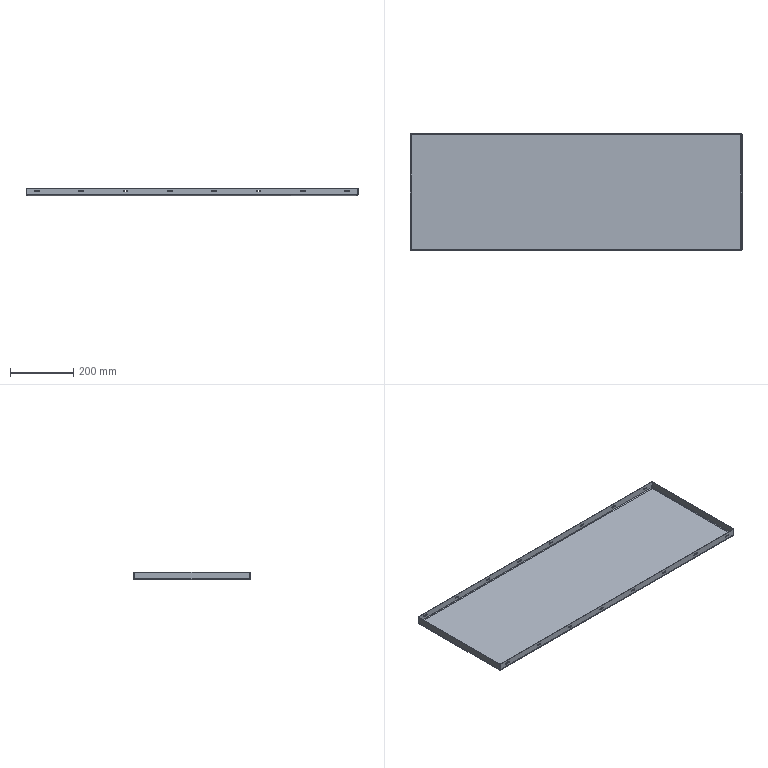Part | SolidWorks | features EdgeFlange 1, FlatPattern 1, ICE 1, SMBaseFlange 1, SheetMetal 1 | 1 solid | 102 faces | box 1048 x 368 x 25 mm | volume 891323 mm3 | plane 54 | cylinder 40 | spline 8 | commonest cylinder face diameters 4.5 x32 4 x4 8 x4